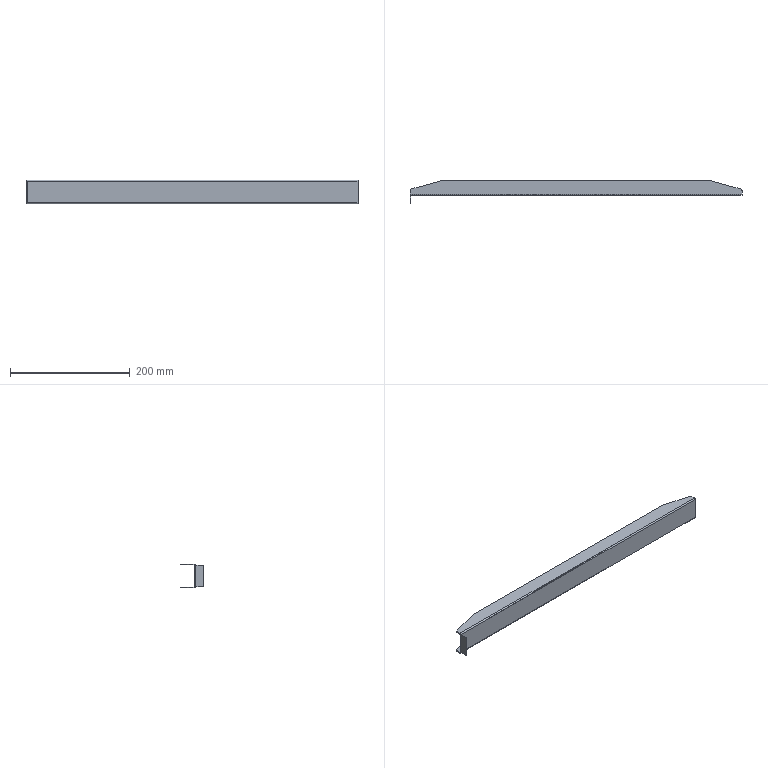Part | 1 solid | 44 faces | box 555 x 38.8 x 40 mm | volume 56167 mm3 | plane 30 | cylinder 14 | commonest cylinder face diameters 4 x8 1.48 x3 3.88 x3
STEP:
#1=CARTESIAN_POINT('',(-275.56,0.,18.06));
#2=VERTEX_POINT('',#1);
#3=CARTESIAN_POINT('',(-277.5,0.,18.06));
#4=VERTEX_POINT('',#3);
#5=CARTESIAN_POINT('',(277.5,0.,18.06));
#6=DIRECTION('',(-1.,0.,0.));
#7=VECTOR('',#6,1000.);
#8=LINE('',#5,#7);
#9=EDGE_CURVE('',#2,#4,#8,.T.);
#10=ORIENTED_EDGE('',*,*,#9,.F.);
#11=CARTESIAN_POINT('',(-277.353,-1.2,18.06));
#12=VERTEX_POINT('',#11);
#13=CARTESIAN_POINT('',(-275.56,-1.94,18.06));
#14=DIRECTION('',(0.,0.,1.));
#15=DIRECTION('',(-1.,0.,0.));
#16=AXIS2_PLACEMENT_3D('',#13,#14,#15);
#17=CIRCLE('',#16,1.94);
#18=EDGE_CURVE('',#2,#12,#17,.T.);
#19=ORIENTED_EDGE('',*,*,#18,.T.);
#20=CARTESIAN_POINT('',(-277.5,-1.2,18.06));
#21=VERTEX_POINT('',#20);
#22=CARTESIAN_POINT('',(-275.56,-1.2,18.06));
#23=DIRECTION('',(-1.,0.,0.));
#24=VECTOR('',#23,1000.);
#25=LINE('',#22,#24);
#26=EDGE_CURVE('',#12,#21,#25,.T.);
#27=ORIENTED_EDGE('',*,*,#26,.T.);
#28=CARTESIAN_POINT('',(-277.5,0.,18.06));
#29=DIRECTION('',(0.,-1.,0.));
#30=VECTOR('',#29,1000.);
#31=LINE('',#28,#30);
#32=EDGE_CURVE('',#4,#21,#31,.T.);
#33=ORIENTED_EDGE('',*,*,#32,.F.);
#34=EDGE_LOOP('',(#10,#19,#27,#33));
#35=FACE_OUTER_BOUND('',#34,.T.);
#36=CARTESIAN_POINT('',(-275.56,-1.2,18.06));
#37=DIRECTION('',(0.,0.,-1.));
#38=DIRECTION('',(-1.,0.,0.));
#39=AXIS2_PLACEMENT_3D('',#36,#37,#38);
#40=PLANE('',#39);
#41=ADVANCED_FACE('',(#35),#40,.T.);
#42=CARTESIAN_POINT('',(-277.5,-1.2,-18.06));
#43=VERTEX_POINT('',#42);
#44=CARTESIAN_POINT('',(-277.353,-1.2,-18.06));
#45=VERTEX_POINT('',#44);
#46=CARTESIAN_POINT('',(-277.5,-1.2,-18.06));
#47=DIRECTION('',(1.,0.,0.));
#48=VECTOR('',#47,1000.);
#49=LINE('',#46,#48);
#50=EDGE_CURVE('',#43,#45,#49,.T.);
#51=ORIENTED_EDGE('',*,*,#50,.T.);
#52=CARTESIAN_POINT('',(-275.56,0.,-18.06));
#53=VERTEX_POINT('',#52);
#54=CARTESIAN_POINT('',(-275.56,-1.94,-18.06));
#55=DIRECTION('',(0.,0.,-1.));
#56=DIRECTION('',(-1.,0.,0.));
#57=AXIS2_PLACEMENT_3D('',#54,#55,#56);
#58=CIRCLE('',#57,1.94);
#59=EDGE_CURVE('',#45,#53,#58,.T.);
#60=ORIENTED_EDGE('',*,*,#59,.T.);
#61=CARTESIAN_POINT('',(-277.5,0.,-18.06));
#62=VERTEX_POINT('',#61);
#63=CARTESIAN_POINT('',(-277.5,0.,-18.06));
#64=DIRECTION('',(1.,0.,0.));
#65=VECTOR('',#64,1000.);
#66=LINE('',#63,#65);
#67=EDGE_CURVE('',#62,#53,#66,.T.);
#68=ORIENTED_EDGE('',*,*,#67,.F.);
#69=CARTESIAN_POINT('',(-277.5,0.,-18.06));
#70=DIRECTION('',(0.,-1.,0.));
#71=VECTOR('',#70,1000.);
#72=LINE('',#69,#71);
#73=EDGE_CURVE('',#62,#43,#72,.T.);
#74=ORIENTED_EDGE('',*,*,#73,.T.);
#75=EDGE_LOOP('',(#51,#60,#68,#74));
#76=FACE_OUTER_BOUND('',#75,.T.);
#77=CARTESIAN_POINT('',(-277.5,-1.2,-18.06));
#78=DIRECTION('',(0.,0.,1.));
#79=DIRECTION('',(1.,0.,0.));
#80=AXIS2_PLACEMENT_3D('',#77,#78,#79);
#81=PLANE('',#80);
#82=ADVANCED_FACE('',(#76),#81,.T.);
#83=CARTESIAN_POINT('',(277.5,-1.2,18.06));
#84=VERTEX_POINT('',#83);
#85=CARTESIAN_POINT('',(-275.56,-1.2,18.06));
#86=VERTEX_POINT('',#85);
#87=CARTESIAN_POINT('',(277.5,-1.2,18.06));
#88=DIRECTION('',(-1.,0.,0.));
#89=VECTOR('',#88,1000.);
#90=LINE('',#87,#89);
#91=EDGE_CURVE('',#84,#86,#90,.T.);
#92=ORIENTED_EDGE('',*,*,#91,.T.);
#93=CARTESIAN_POINT('',(-275.56,-1.2,-18.06));
#94=VERTEX_POINT('',#93);
#95=CARTESIAN_POINT('',(-275.56,-1.2,-18.06));
#96=DIRECTION('',(0.,0.,1.));
#97=VECTOR('',#96,1000.);
#98=LINE('',#95,#97);
#99=EDGE_CURVE('',#94,#86,#98,.T.);
#100=ORIENTED_EDGE('',*,*,#99,.F.);
#101=CARTESIAN_POINT('',(277.5,-1.2,-18.06));
#102=VERTEX_POINT('',#101);
#103=CARTESIAN_POINT('',(-277.5,-1.2,-18.06));
#104=DIRECTION('',(1.,0.,0.));
#105=VECTOR('',#104,1000.);
#106=LINE('',#103,#105);
#107=EDGE_CURVE('',#94,#102,#106,.T.);
#108=ORIENTED_EDGE('',*,*,#107,.T.);
#109=CARTESIAN_POINT('',(277.5,-1.2,20.));
#110=DIRECTION('',(0.,0.,-1.));
#111=VECTOR('',#110,1000.);
#112=LINE('',#109,#111);
#113=EDGE_CURVE('',#84,#102,#112,.T.);
#114=ORIENTED_EDGE('',*,*,#113,.F.);
#115=EDGE_LOOP('',(#92,#100,#108,#114));
#116=FACE_OUTER_BOUND('',#115,.T.);
#117=CARTESIAN_POINT('',(0.,-1.2,0.));
#118=DIRECTION('',(0.,-1.,0.));
#119=DIRECTION('',(0.,0.,-1.));
#120=AXIS2_PLACEMENT_3D('',#117,#118,#119);
#121=PLANE('',#120);
#122=ADVANCED_FACE('',(#116),#121,.T.);
#123=CARTESIAN_POINT('',(-275.56,0.,-18.06));
#124=DIRECTION('',(0.,0.,1.));
#125=VECTOR('',#124,1000.);
#126=LINE('',#123,#125);
#127=EDGE_CURVE('',#53,#2,#126,.T.);
#128=ORIENTED_EDGE('',*,*,#127,.T.);
#129=CARTESIAN_POINT('',(277.5,0.,18.06));
#130=VERTEX_POINT('',#129);
#131=CARTESIAN_POINT('',(277.5,0.,18.06));
#132=DIRECTION('',(-1.,0.,0.));
#133=VECTOR('',#132,1000.);
#134=LINE('',#131,#133);
#135=EDGE_CURVE('',#130,#2,#134,.T.);
#136=ORIENTED_EDGE('',*,*,#135,.F.);
#137=CARTESIAN_POINT('',(277.5,0.,-18.06));
#138=VERTEX_POINT('',#137);
#139=CARTESIAN_POINT('',(277.5,0.,20.));
#140=DIRECTION('',(0.,0.,-1.));
#141=VECTOR('',#140,1000.);
#142=LINE('',#139,#141);
#143=EDGE_CURVE('',#130,#138,#142,.T.);
#144=ORIENTED_EDGE('',*,*,#143,.T.);
#145=CARTESIAN_POINT('',(-277.5,0.,-18.06));
#146=DIRECTION('',(1.,0.,0.));
#147=VECTOR('',#146,1000.);
#148=LINE('',#145,#147);
#149=EDGE_CURVE('',#53,#138,#148,.T.);
#150=ORIENTED_EDGE('',*,*,#149,.F.);
#151=EDGE_LOOP('',(#128,#136,#144,#150));
#152=FACE_OUTER_BOUND('',#151,.T.);
#153=CARTESIAN_POINT('',(0.,0.,0.));
#154=DIRECTION('',(0.,-1.,0.));
#155=DIRECTION('',(0.,0.,-1.));
#156=AXIS2_PLACEMENT_3D('',#153,#154,#155);
#157=PLANE('',#156);
#158=ADVANCED_FACE('',(#152),#157,.F.);
#159=CARTESIAN_POINT('',(277.5,0.,-18.06));
#160=DIRECTION('',(0.,-1.,0.));
#161=VECTOR('',#160,1000.);
#162=LINE('',#159,#161);
#163=EDGE_CURVE('',#138,#102,#162,.T.);
#164=ORIENTED_EDGE('',*,*,#163,.F.);
#165=ORIENTED_EDGE('',*,*,#143,.F.);
#166=CARTESIAN_POINT('',(277.5,0.,18.06));
#167=DIRECTION('',(0.,-1.,0.));
#168=VECTOR('',#167,1000.);
#169=LINE('',#166,#168);
#170=EDGE_CURVE('',#130,#84,#169,.T.);
#171=ORIENTED_EDGE('',*,*,#170,.T.);
#172=ORIENTED_EDGE('',*,*,#113,.T.);
#173=EDGE_LOOP('',(#164,#165,#171,#172));
#174=FACE_OUTER_BOUND('',#173,.T.);
#175=CARTESIAN_POINT('',(277.5,-1.2,20.));
#176=DIRECTION('',(1.,0.,0.));
#177=DIRECTION('',(0.,0.,-1.));
#178=AXIS2_PLACEMENT_3D('',#175,#176,#177);
#179=PLANE('',#178);
#180=ADVANCED_FACE('',(#174),#179,.T.);
#181=CARTESIAN_POINT('',(-277.5,0.74,18.8));
#182=VERTEX_POINT('',#181);
#183=CARTESIAN_POINT('',(-277.5,0.74,20.));
#184=VERTEX_POINT('',#183);
#185=CARTESIAN_POINT('',(-277.5,0.74,20.));
#186=DIRECTION('',(0.,0.,1.));
#187=VECTOR('',#186,1000.);
#188=LINE('',#185,#187);
#189=EDGE_CURVE('',#182,#184,#188,.T.);
#190=ORIENTED_EDGE('',*,*,#189,.F.);
#191=CARTESIAN_POINT('',(-277.5,0.74,18.06));
#192=DIRECTION('',(-1.,0.,0.));
#193=DIRECTION('',(0.,0.,-1.));
#194=AXIS2_PLACEMENT_3D('',#191,#192,#193);
#195=CIRCLE('',#194,0.74);
#196=EDGE_CURVE('',#4,#182,#195,.T.);
#197=ORIENTED_EDGE('',*,*,#196,.F.);
#198=ORIENTED_EDGE('',*,*,#32,.T.);
#199=CARTESIAN_POINT('',(-277.5,0.74,18.06));
#200=DIRECTION('',(-1.,0.,0.));
#201=DIRECTION('',(0.,0.,-1.));
#202=AXIS2_PLACEMENT_3D('',#199,#200,#201);
#203=CIRCLE('',#202,1.94);
#204=EDGE_CURVE('',#21,#184,#203,.T.);
#205=ORIENTED_EDGE('',*,*,#204,.T.);
#206=EDGE_LOOP('',(#190,#197,#198,#205));
#207=FACE_OUTER_BOUND('',#206,.T.);
#208=CARTESIAN_POINT('',(-277.5,0.74,18.06));
#209=DIRECTION('',(-1.,0.,0.));
#210=DIRECTION('',(0.,0.,1.));
#211=AXIS2_PLACEMENT_3D('',#208,#209,#210);
#212=PLANE('',#211);
#213=ADVANCED_FACE('',(#207),#212,.T.);
#214=CARTESIAN_POINT('',(277.5,0.74,18.8));
#215=VERTEX_POINT('',#214);
#216=CARTESIAN_POINT('',(277.5,0.74,18.06));
#217=DIRECTION('',(1.,0.,0.));
#218=DIRECTION('',(0.,0.,-1.));
#219=AXIS2_PLACEMENT_3D('',#216,#217,#218);
#220=CIRCLE('',#219,0.74);
#221=EDGE_CURVE('',#215,#130,#220,.T.);
#222=ORIENTED_EDGE('',*,*,#221,.F.);
#223=CARTESIAN_POINT('',(277.5,0.74,20.));
#224=VERTEX_POINT('',#223);
#225=CARTESIAN_POINT('',(277.5,0.74,18.8));
#226=DIRECTION('',(0.,0.,1.));
#227=VECTOR('',#226,1000.);
#228=LINE('',#225,#227);
#229=EDGE_CURVE('',#215,#224,#228,.T.);
#230=ORIENTED_EDGE('',*,*,#229,.T.);
#231=CARTESIAN_POINT('',(277.5,0.74,18.06));
#232=DIRECTION('',(1.,0.,0.));
#233=DIRECTION('',(0.,0.,-1.));
#234=AXIS2_PLACEMENT_3D('',#231,#232,#233);
#235=CIRCLE('',#234,1.94);
#236=EDGE_CURVE('',#224,#84,#235,.T.);
#237=ORIENTED_EDGE('',*,*,#236,.T.);
#238=ORIENTED_EDGE('',*,*,#170,.F.);
#239=EDGE_LOOP('',(#222,#230,#237,#238));
#240=FACE_OUTER_BOUND('',#239,.T.);
#241=CARTESIAN_POINT('',(277.5,0.74,18.06));
#242=DIRECTION('',(-1.,0.,0.));
#243=DIRECTION('',(0.,0.,1.));
#244=AXIS2_PLACEMENT_3D('',#241,#242,#243);
#245=PLANE('',#244);
#246=ADVANCED_FACE('',(#240),#245,.F.);
#247=ORIENTED_EDGE('',*,*,#91,.F.);
#248=ORIENTED_EDGE('',*,*,#236,.F.);
#249=CARTESIAN_POINT('',(0.,0.74,20.));
#250=DIRECTION('',(1.,0.,0.));
#251=VECTOR('',#250,1000.);
#252=LINE('',#249,#251);
#253=EDGE_CURVE('',#184,#224,#252,.T.);
#254=ORIENTED_EDGE('',*,*,#253,.F.);
#255=ORIENTED_EDGE('',*,*,#204,.F.);
#256=ORIENTED_EDGE('',*,*,#26,.F.);
#257=CARTESIAN_POINT('',(-275.56,-1.2,18.06));
#258=DIRECTION('',(-1.,0.,0.));
#259=VECTOR('',#258,1000.);
#260=LINE('',#257,#259);
#261=EDGE_CURVE('',#86,#12,#260,.T.);
#262=ORIENTED_EDGE('',*,*,#261,.F.);
#263=EDGE_LOOP('',(#247,#248,#254,#255,#256,#262));
#264=FACE_OUTER_BOUND('',#263,.T.);
#265=CARTESIAN_POINT('',(277.5,0.74,18.06));
#266=DIRECTION('',(1.,0.,0.));
#267=DIRECTION('',(0.,0.,1.));
#268=AXIS2_PLACEMENT_3D('',#265,#266,#267);
#269=CYLINDRICAL_SURFACE('',#268,1.94);
#270=ADVANCED_FACE('',(#264),#269,.T.);
#271=ORIENTED_EDGE('',*,*,#135,.T.);
#272=ORIENTED_EDGE('',*,*,#9,.T.);
#273=ORIENTED_EDGE('',*,*,#196,.T.);
#274=CARTESIAN_POINT('',(-277.5,0.74,18.8));
#275=DIRECTION('',(1.,0.,0.));
#276=VECTOR('',#275,1000.);
#277=LINE('',#274,#276);
#278=EDGE_CURVE('',#182,#215,#277,.T.);
#279=ORIENTED_EDGE('',*,*,#278,.T.);
#280=ORIENTED_EDGE('',*,*,#221,.T.);
#281=EDGE_LOOP('',(#271,#272,#273,#279,#280));
#282=FACE_OUTER_BOUND('',#281,.T.);
#283=CARTESIAN_POINT('',(277.5,0.74,18.06));
#284=DIRECTION('',(1.,0.,0.));
#285=DIRECTION('',(0.,0.,1.));
#286=AXIS2_PLACEMENT_3D('',#283,#284,#285);
#287=CYLINDRICAL_SURFACE('',#286,0.74);
#288=ADVANCED_FACE('',(#282),#287,.F.);
#289=CARTESIAN_POINT('',(277.5,7.272,18.8));
#290=VERTEX_POINT('',#289);
#291=CARTESIAN_POINT('',(277.5,0.,18.8));
#292=DIRECTION('',(0.,-1.,0.));
#293=VECTOR('',#292,1000.);
#294=LINE('',#291,#293);
#295=EDGE_CURVE('',#290,#215,#294,.T.);
#296=ORIENTED_EDGE('',*,*,#295,.F.);
#297=CARTESIAN_POINT('',(277.5,7.272,20.));
#298=VERTEX_POINT('',#297);
#299=CARTESIAN_POINT('',(277.5,7.272,20.));
#300=DIRECTION('',(0.,0.,1.));
#301=VECTOR('',#300,1000.);
#302=LINE('',#299,#301);
#303=EDGE_CURVE('',#290,#298,#302,.T.);
#304=ORIENTED_EDGE('',*,*,#303,.T.);
#305=CARTESIAN_POINT('',(277.5,0.,20.));
#306=DIRECTION('',(0.,-1.,0.));
#307=VECTOR('',#306,1000.);
#308=LINE('',#305,#307);
#309=EDGE_CURVE('',#298,#224,#308,.T.);
#310=ORIENTED_EDGE('',*,*,#309,.T.);
#311=ORIENTED_EDGE('',*,*,#229,.F.);
#312=EDGE_LOOP('',(#296,#304,#310,#311));
#313=FACE_OUTER_BOUND('',#312,.T.);
#314=CARTESIAN_POINT('',(277.5,0.,20.));
#315=DIRECTION('',(1.,0.,0.));
#316=DIRECTION('',(0.,0.,-1.));
#317=AXIS2_PLACEMENT_3D('',#314,#315,#316);
#318=PLANE('',#317);
#319=ADVANCED_FACE('',(#313),#318,.T.);
#320=CARTESIAN_POINT('',(-277.5,7.272,20.));
#321=VERTEX_POINT('',#320);
#322=CARTESIAN_POINT('',(-277.5,23.8,20.));
#323=DIRECTION('',(0.,1.,0.));
#324=VECTOR('',#323,1000.);
#325=LINE('',#322,#324);
#326=EDGE_CURVE('',#184,#321,#325,.T.);
#327=ORIENTED_EDGE('',*,*,#326,.T.);
#328=CARTESIAN_POINT('',(-277.5,7.272,18.8));
#329=VERTEX_POINT('',#328);
#330=CARTESIAN_POINT('',(-277.5,7.272,20.));
#331=DIRECTION('',(0.,0.,-1.));
#332=VECTOR('',#331,1000.);
#333=LINE('',#330,#332);
#334=EDGE_CURVE('',#321,#329,#333,.T.);
#335=ORIENTED_EDGE('',*,*,#334,.T.);
#336=CARTESIAN_POINT('',(-277.5,0.,18.8));
#337=DIRECTION('',(0.,1.,0.));
#338=VECTOR('',#337,1000.);
#339=LINE('',#336,#338);
#340=EDGE_CURVE('',#182,#329,#339,.T.);
#341=ORIENTED_EDGE('',*,*,#340,.F.);
#342=ORIENTED_EDGE('',*,*,#189,.T.);
#343=EDGE_LOOP('',(#327,#335,#341,#342));
#344=FACE_OUTER_BOUND('',#343,.T.);
#345=CARTESIAN_POINT('',(-277.5,23.8,20.));
#346=DIRECTION('',(-1.,0.,0.));
#347=DIRECTION('',(0.,0.,1.));
#348=AXIS2_PLACEMENT_3D('',#345,#346,#347);
#349=PLANE('',#348);
#350=ADVANCED_FACE('',(#344),#349,.T.);
#351=CARTESIAN_POINT('',(-222.758,23.73,20.));
#352=VERTEX_POINT('',#351);
#353=CARTESIAN_POINT('',(-276.026,9.202,20.));
#354=VERTEX_POINT('',#353);
#355=CARTESIAN_POINT('',(-21.445,78.633,20.));
#356=DIRECTION('',(-0.9648,-0.2631,0.));
#357=VECTOR('',#356,1000.);
#358=LINE('',#355,#357);
#359=EDGE_CURVE('',#352,#354,#358,.T.);
#360=ORIENTED_EDGE('',*,*,#359,.T.);
#361=CARTESIAN_POINT('',(-275.5,7.272,20.));
#362=DIRECTION('',(0.,0.,1.));
#363=DIRECTION('',(0.,-1.,0.));
#364=AXIS2_PLACEMENT_3D('',#361,#362,#363);
#365=CIRCLE('',#364,2.);
#366=EDGE_CURVE('',#354,#321,#365,.T.);
#367=ORIENTED_EDGE('',*,*,#366,.T.);
#368=ORIENTED_EDGE('',*,*,#326,.F.);
#369=ORIENTED_EDGE('',*,*,#253,.T.);
#370=ORIENTED_EDGE('',*,*,#309,.F.);
#371=CARTESIAN_POINT('',(276.026,9.202,20.));
#372=VERTEX_POINT('',#371);
#373=CARTESIAN_POINT('',(275.5,7.272,20.));
#374=DIRECTION('',(0.,0.,1.));
#375=DIRECTION('',(0.,-1.,0.));
#376=AXIS2_PLACEMENT_3D('',#373,#374,#375);
#377=CIRCLE('',#376,2.);
#378=EDGE_CURVE('',#298,#372,#377,.T.);
#379=ORIENTED_EDGE('',*,*,#378,.T.);
#380=CARTESIAN_POINT('',(222.758,23.73,20.));
#381=VERTEX_POINT('',#380);
#382=CARTESIAN_POINT('',(21.445,78.633,20.));
#383=DIRECTION('',(-0.9648,0.2631,0.));
#384=VECTOR('',#383,1000.);
#385=LINE('',#382,#384);
#386=EDGE_CURVE('',#372,#381,#385,.T.);
#387=ORIENTED_EDGE('',*,*,#386,.T.);
#388=CARTESIAN_POINT('',(222.232,23.8,20.));
#389=VERTEX_POINT('',#388);
#390=CARTESIAN_POINT('',(222.232,21.8,20.));
#391=DIRECTION('',(0.,0.,1.));
#392=DIRECTION('',(0.,-1.,0.));
#393=AXIS2_PLACEMENT_3D('',#390,#391,#392);
#394=CIRCLE('',#393,2.);
#395=EDGE_CURVE('',#381,#389,#394,.T.);
#396=ORIENTED_EDGE('',*,*,#395,.T.);
#397=CARTESIAN_POINT('',(-222.232,23.8,20.));
#398=VERTEX_POINT('',#397);
#399=CARTESIAN_POINT('',(277.5,23.8,20.));
#400=DIRECTION('',(1.,0.,0.));
#401=VECTOR('',#400,1000.);
#402=LINE('',#399,#401);
#403=EDGE_CURVE('',#398,#389,#402,.T.);
#404=ORIENTED_EDGE('',*,*,#403,.F.);
#405=CARTESIAN_POINT('',(-222.232,21.8,20.));
#406=DIRECTION('',(0.,0.,1.));
#407=DIRECTION('',(0.,-1.,0.));
#408=AXIS2_PLACEMENT_3D('',#405,#406,#407);
#409=CIRCLE('',#408,2.);
#410=EDGE_CURVE('',#398,#352,#409,.T.);
#411=ORIENTED_EDGE('',*,*,#410,.T.);
#412=EDGE_LOOP('',(#360,#367,#368,#369,#370,#379,#387,#396,#404,#411));
#413=FACE_OUTER_BOUND('',#412,.T.);
#414=CARTESIAN_POINT('',(0.,0.,20.));
#415=DIRECTION('',(0.,0.,1.));
#416=DIRECTION('',(0.,-1.,0.));
#417=AXIS2_PLACEMENT_3D('',#414,#415,#416);
#418=PLANE('',#417);
#419=ADVANCED_FACE('',(#413),#418,.T.);
#420=ORIENTED_EDGE('',*,*,#340,.T.);
#421=CARTESIAN_POINT('',(-276.026,9.202,18.8));
#422=VERTEX_POINT('',#421);
#423=CARTESIAN_POINT('',(-275.5,7.272,18.8));
#424=DIRECTION('',(0.,0.,-1.));
#425=DIRECTION('',(0.,-1.,0.));
#426=AXIS2_PLACEMENT_3D('',#423,#424,#425);
#427=CIRCLE('',#426,2.);
#428=EDGE_CURVE('',#329,#422,#427,.T.);
#429=ORIENTED_EDGE('',*,*,#428,.T.);
#430=CARTESIAN_POINT('',(-222.758,23.73,18.8));
#431=VERTEX_POINT('',#430);
#432=CARTESIAN_POINT('',(-277.5,8.8,18.8));
#433=DIRECTION('',(0.9648,0.2631,0.));
#434=VECTOR('',#433,1000.);
#435=LINE('',#432,#434);
#436=EDGE_CURVE('',#422,#431,#435,.T.);
#437=ORIENTED_EDGE('',*,*,#436,.T.);
#438=CARTESIAN_POINT('',(-222.232,23.8,18.8));
#439=VERTEX_POINT('',#438);
#440=CARTESIAN_POINT('',(-222.232,21.8,18.8));
#441=DIRECTION('',(0.,0.,-1.));
#442=DIRECTION('',(0.,-1.,0.));
#443=AXIS2_PLACEMENT_3D('',#440,#441,#442);
#444=CIRCLE('',#443,2.);
#445=EDGE_CURVE('',#431,#439,#444,.T.);
#446=ORIENTED_EDGE('',*,*,#445,.T.);
#447=CARTESIAN_POINT('',(222.232,23.8,18.8));
#448=VERTEX_POINT('',#447);
#449=CARTESIAN_POINT('',(0.,23.8,18.8));
#450=DIRECTION('',(1.,0.,0.));
#451=VECTOR('',#450,1000.);
#452=LINE('',#449,#451);
#453=EDGE_CURVE('',#439,#448,#452,.T.);
#454=ORIENTED_EDGE('',*,*,#453,.T.);
#455=CARTESIAN_POINT('',(222.758,23.73,18.8));
#456=VERTEX_POINT('',#455);
#457=CARTESIAN_POINT('',(222.232,21.8,18.8));
#458=DIRECTION('',(0.,0.,-1.));
#459=DIRECTION('',(0.,-1.,0.));
#460=AXIS2_PLACEMENT_3D('',#457,#458,#459);
#461=CIRCLE('',#460,2.);
#462=EDGE_CURVE('',#448,#456,#461,.T.);
#463=ORIENTED_EDGE('',*,*,#462,.T.);
#464=CARTESIAN_POINT('',(276.026,9.202,18.8));
#465=VERTEX_POINT('',#464);
#466=CARTESIAN_POINT('',(222.5,23.8,18.8));
#467=DIRECTION('',(0.9648,-0.2631,0.));
#468=VECTOR('',#467,1000.);
#469=LINE('',#466,#468);
#470=EDGE_CURVE('',#456,#465,#469,.T.);
#471=ORIENTED_EDGE('',*,*,#470,.T.);
#472=CARTESIAN_POINT('',(275.5,7.272,18.8));
#473=DIRECTION('',(0.,0.,-1.));
#474=DIRECTION('',(0.,-1.,0.));
#475=AXIS2_PLACEMENT_3D('',#472,#473,#474);
#476=CIRCLE('',#475,2.);
#477=EDGE_CURVE('',#465,#290,#476,.T.);
#478=ORIENTED_EDGE('',*,*,#477,.T.);
#479=ORIENTED_EDGE('',*,*,#295,.T.);
#480=ORIENTED_EDGE('',*,*,#278,.F.);
#481=EDGE_LOOP('',(#420,#429,#437,#446,#454,#463,#471,#478,#479,#480));
#482=FACE_OUTER_BOUND('',#481,.T.);
#483=CARTESIAN_POINT('',(0.,0.,18.8));
#484=DIRECTION('',(0.,0.,1.));
#485=DIRECTION('',(0.,-1.,0.));
#486=AXIS2_PLACEMENT_3D('',#483,#484,#485);
#487=PLANE('',#486);
#488=ADVANCED_FACE('',(#482),#487,.F.);
#489=ORIENTED_EDGE('',*,*,#453,.F.);
#490=CARTESIAN_POINT('',(-222.232,23.8,20.));
#491=DIRECTION('',(0.,0.,1.));
#492=VECTOR('',#491,1000.);
#493=LINE('',#490,#492);
#494=EDGE_CURVE('',#439,#398,#493,.T.);
#495=ORIENTED_EDGE('',*,*,#494,.T.);
#496=ORIENTED_EDGE('',*,*,#403,.T.);
#497=CARTESIAN_POINT('',(222.232,23.8,20.));
#498=DIRECTION('',(0.,0.,-1.));
#499=VECTOR('',#498,1000.);
#500=LINE('',#497,#499);
#501=EDGE_CURVE('',#389,#448,#500,.T.);
#502=ORIENTED_EDGE('',*,*,#501,.T.);
#503=EDGE_LOOP('',(#489,#495,#496,#502));
#504=FACE_OUTER_BOUND('',#503,.T.);
#505=CARTESIAN_POINT('',(277.5,23.8,20.));
#506=DIRECTION('',(0.,1.,0.));
#507=DIRECTION('',(0.,0.,1.));
#508=AXIS2_PLACEMENT_3D('',#505,#506,#507);
#509=PLANE('',#508);
#510=ADVANCED_FACE('',(#504),#509,.T.);
#511=CARTESIAN_POINT('',(277.5,0.74,-18.8));
#512=VERTEX_POINT('',#511);
#513=CARTESIAN_POINT('',(277.5,0.74,-20.));
#514=VERTEX_POINT('',#513);
#515=CARTESIAN_POINT('',(277.5,0.74,-20.));
#516=DIRECTION('',(0.,0.,-1.));
#517=VECTOR('',#516,1000.);
#518=LINE('',#515,#517);
#519=EDGE_CURVE('',#512,#514,#518,.T.);
#520=ORIENTED_EDGE('',*,*,#519,.F.);
#521=CARTESIAN_POINT('',(277.5,0.74,-18.06));
#522=DIRECTION('',(1.,0.,0.));
#523=DIRECTION('',(0.,0.,1.));
#524=AXIS2_PLACEMENT_3D('',#521,#522,#523);
#525=CIRCLE('',#524,0.74);
#526=EDGE_CURVE('',#138,#512,#525,.T.);
#527=ORIENTED_EDGE('',*,*,#526,.F.);
#528=ORIENTED_EDGE('',*,*,#163,.T.);
#529=CARTESIAN_POINT('',(277.5,0.74,-18.06));
#530=DIRECTION('',(1.,0.,0.));
#531=DIRECTION('',(0.,0.,1.));
#532=AXIS2_PLACEMENT_3D('',#529,#530,#531);
#533=CIRCLE('',#532,1.94);
#534=EDGE_CURVE('',#102,#514,#533,.T.);
#535=ORIENTED_EDGE('',*,*,#534,.T.);
#536=EDGE_LOOP('',(#520,#527,#528,#535));
#537=FACE_OUTER_BOUND('',#536,.T.);
#538=CARTESIAN_POINT('',(277.5,0.74,-18.06));
#539=DIRECTION('',(1.,0.,0.));
#540=DIRECTION('',(0.,0.,-1.));
#541=AXIS2_PLACEMENT_3D('',#538,#539,#540);
#542=PLANE('',#541);
#543=ADVANCED_FACE('',(#537),#542,.T.);
#544=CARTESIAN_POINT('',(-277.5,0.74,-18.8));
#545=VERTEX_POINT('',#544);
#546=CARTESIAN_POINT('',(-277.5,0.74,-18.06));
#547=DIRECTION('',(-1.,0.,0.));
#548=DIRECTION('',(0.,0.,1.));
#549=AXIS2_PLACEMENT_3D('',#546,#547,#548);
#550=CIRCLE('',#549,0.74);
#551=EDGE_CURVE('',#545,#62,#550,.T.);
#552=ORIENTED_EDGE('',*,*,#551,.F.);
#553=CARTESIAN_POINT('',(-277.5,0.74,-20.));
#554=VERTEX_POINT('',#553);
#555=CARTESIAN_POINT('',(-277.5,0.74,-18.8));
#556=DIRECTION('',(0.,0.,-1.));
#557=VECTOR('',#556,1000.);
#558=LINE('',#555,#557);
#559=EDGE_CURVE('',#545,#554,#558,.T.);
#560=ORIENTED_EDGE('',*,*,#559,.T.);
#561=CARTESIAN_POINT('',(-277.5,0.74,-18.06));
#562=DIRECTION('',(-1.,0.,0.));
#563=DIRECTION('',(0.,0.,1.));
#564=AXIS2_PLACEMENT_3D('',#561,#562,#563);
#565=CIRCLE('',#564,1.94);
#566=EDGE_CURVE('',#554,#43,#565,.T.);
#567=ORIENTED_EDGE('',*,*,#566,.T.);
#568=ORIENTED_EDGE('',*,*,#73,.F.);
#569=EDGE_LOOP('',(#552,#560,#567,#568));
#570=FACE_OUTER_BOUND('',#569,.T.);
#571=CARTESIAN_POINT('',(-277.5,0.74,-18.06));
#572=DIRECTION('',(1.,0.,0.));
#573=DIRECTION('',(0.,0.,-1.));
#574=AXIS2_PLACEMENT_3D('',#571,#572,#573);
#575=PLANE('',#574);
#576=ADVANCED_FACE('',(#570),#575,.F.);
#577=ORIENTED_EDGE('',*,*,#50,.F.);
#578=ORIENTED_EDGE('',*,*,#566,.F.);
#579=CARTESIAN_POINT('',(277.5,0.74,-20.));
#580=DIRECTION('',(1.,0.,0.));
#581=VECTOR('',#580,1000.);
#582=LINE('',#579,#581);
#583=EDGE_CURVE('',#554,#514,#582,.T.);
#584=ORIENTED_EDGE('',*,*,#583,.T.);
#585=ORIENTED_EDGE('',*,*,#534,.F.);
#586=ORIENTED_EDGE('',*,*,#107,.F.);
#587=CARTESIAN_POINT('',(-277.5,-1.2,-18.06));
#588=DIRECTION('',(1.,0.,0.));
#589=VECTOR('',#588,1000.);
#590=LINE('',#587,#589);
#591=EDGE_CURVE('',#45,#94,#590,.T.);
#592=ORIENTED_EDGE('',*,*,#591,.F.);
#593=EDGE_LOOP('',(#577,#578,#584,#585,#586,#592));
#594=FACE_OUTER_BOUND('',#593,.T.);
#595=CARTESIAN_POINT('',(-277.5,0.74,-18.06));
#596=DIRECTION('',(-1.,0.,0.));
#597=DIRECTION('',(0.,0.,-1.));
#598=AXIS2_PLACEMENT_3D('',#595,#596,#597);
#599=CYLINDRICAL_SURFACE('',#598,1.94);
#600=ADVANCED_FACE('',(#594),#599,.T.);
#601=ORIENTED_EDGE('',*,*,#67,.T.);
#602=ORIENTED_EDGE('',*,*,#149,.T.);
#603=ORIENTED_EDGE('',*,*,#526,.T.);
#604=CARTESIAN_POINT('',(277.5,0.74,-18.8));
#605=DIRECTION('',(-1.,0.,0.));
#606=VECTOR('',#605,1000.);
#607=LINE('',#604,#606);
#608=EDGE_CURVE('',#512,#545,#607,.T.);
#609=ORIENTED_EDGE('',*,*,#608,.T.);
#610=ORIENTED_EDGE('',*,*,#551,.T.);
#611=EDGE_LOOP('',(#601,#602,#603,#609,#610));
#612=FACE_OUTER_BOUND('',#611,.T.);
#613=CARTESIAN_POINT('',(-277.5,0.74,-18.06));
#614=DIRECTION('',(-1.,0.,0.));
#615=DIRECTION('',(0.,0.,-1.));
#616=AXIS2_PLACEMENT_3D('',#613,#614,#615);
#617=CYLINDRICAL_SURFACE('',#616,0.74);
#618=ADVANCED_FACE('',(#612),#617,.F.);
#619=CARTESIAN_POINT('',(277.5,7.272,-20.));
#620=VERTEX_POINT('',#619);
#621=CARTESIAN_POINT('',(277.5,0.,-20.));
#622=DIRECTION('',(0.,1.,0.));
#623=VECTOR('',#622,1000.);
#624=LINE('',#621,#623);
#625=EDGE_CURVE('',#514,#620,#624,.T.);
#626=ORIENTED_EDGE('',*,*,#625,.T.);
#627=CARTESIAN_POINT('',(277.5,7.272,-18.8));
#628=VERTEX_POINT('',#627);
#629=CARTESIAN_POINT('',(277.5,7.272,-20.));
#630=DIRECTION('',(0.,0.,1.));
#631=VECTOR('',#630,1000.);
#632=LINE('',#629,#631);
#633=EDGE_CURVE('',#620,#628,#632,.T.);
#634=ORIENTED_EDGE('',*,*,#633,.T.);
#635=CARTESIAN_POINT('',(277.5,0.,-18.8));
#636=DIRECTION('',(0.,1.,0.));
#637=VECTOR('',#636,1000.);
#638=LINE('',#635,#637);
#639=EDGE_CURVE('',#512,#628,#638,.T.);
#640=ORIENTED_EDGE('',*,*,#639,.F.);
#641=ORIENTED_EDGE('',*,*,#519,.T.);
#642=EDGE_LOOP('',(#626,#634,#640,#641));
#643=FACE_OUTER_BOUND('',#642,.T.);
#644=CARTESIAN_POINT('',(277.5,0.,-20.));
#645=DIRECTION('',(1.,0.,0.));
#646=DIRECTION('',(0.,0.,-1.));
#647=AXIS2_PLACEMENT_3D('',#644,#645,#646);
#648=PLANE('',#647);
#649=ADVANCED_FACE('',(#643),#648,.T.);
#650=CARTESIAN_POINT('',(-277.5,7.272,-18.8));
#651=VERTEX_POINT('',#650);
#652=CARTESIAN_POINT('',(-277.5,0.,-18.8));
#653=DIRECTION('',(0.,-1.,0.));
#654=VECTOR('',#653,1000.);
#655=LINE('',#652,#654);
#656=EDGE_CURVE('',#651,#545,#655,.T.);
#657=ORIENTED_EDGE('',*,*,#656,.F.);
#658=CARTESIAN_POINT('',(-277.5,7.272,-20.));
#659=VERTEX_POINT('',#658);
#660=CARTESIAN_POINT('',(-277.5,7.272,-20.));
#661=DIRECTION('',(0.,0.,-1.));
#662=VECTOR('',#661,1000.);
#663=LINE('',#660,#662);
#664=EDGE_CURVE('',#651,#659,#663,.T.);
#665=ORIENTED_EDGE('',*,*,#664,.T.);
#666=CARTESIAN_POINT('',(-277.5,23.8,-20.));
#667=DIRECTION('',(0.,-1.,0.));
#668=VECTOR('',#667,1000.);
#669=LINE('',#666,#668);
#670=EDGE_CURVE('',#659,#554,#669,.T.);
#671=ORIENTED_EDGE('',*,*,#670,.T.);
#672=ORIENTED_EDGE('',*,*,#559,.F.);
#673=EDGE_LOOP('',(#657,#665,#671,#672));
#674=FACE_OUTER_BOUND('',#673,.T.);
#675=CARTESIAN_POINT('',(-277.5,23.8,-20.));
#676=DIRECTION('',(-1.,0.,0.));
#677=DIRECTION('',(0.,0.,1.));
#678=AXIS2_PLACEMENT_3D('',#675,#676,#677);
#679=PLANE('',#678);
#680=ADVANCED_FACE('',(#674),#679,.T.);
#681=CARTESIAN_POINT('',(222.758,23.73,-20.));
#682=VERTEX_POINT('',#681);
#683=CARTESIAN_POINT('',(276.026,9.202,-20.));
#684=VERTEX_POINT('',#683);
#685=CARTESIAN_POINT('',(277.5,8.8,-20.));
#686=DIRECTION('',(0.9648,-0.2631,0.));
#687=VECTOR('',#686,1000.);
#688=LINE('',#685,#687);
#689=EDGE_CURVE('',#682,#684,#688,.T.);
#690=ORIENTED_EDGE('',*,*,#689,.T.);
#691=CARTESIAN_POINT('',(275.5,7.272,-20.));
#692=DIRECTION('',(0.,0.,-1.));
#693=DIRECTION('',(1.,0.,0.));
#694=AXIS2_PLACEMENT_3D('',#691,#692,#693);
#695=CIRCLE('',#694,2.);
#696=EDGE_CURVE('',#684,#620,#695,.T.);
#697=ORIENTED_EDGE('',*,*,#696,.T.);
#698=ORIENTED_EDGE('',*,*,#625,.F.);
#699=ORIENTED_EDGE('',*,*,#583,.F.);
#700=ORIENTED_EDGE('',*,*,#670,.F.);
#701=CARTESIAN_POINT('',(-276.026,9.202,-20.));
#702=VERTEX_POINT('',#701);
#703=CARTESIAN_POINT('',(-275.5,7.272,-20.));
#704=DIRECTION('',(0.,0.,-1.));
#705=DIRECTION('',(1.,0.,0.));
#706=AXIS2_PLACEMENT_3D('',#703,#704,#705);
#707=CIRCLE('',#706,2.);
#708=EDGE_CURVE('',#659,#702,#707,.T.);
#709=ORIENTED_EDGE('',*,*,#708,.T.);
#710=CARTESIAN_POINT('',(-222.758,23.73,-20.));
#711=VERTEX_POINT('',#710);
#712=CARTESIAN_POINT('',(-222.5,23.8,-20.));
#713=DIRECTION('',(0.9648,0.2631,0.));
#714=VECTOR('',#713,1000.);
#715=LINE('',#712,#714);
#716=EDGE_CURVE('',#702,#711,#715,.T.);
#717=ORIENTED_EDGE('',*,*,#716,.T.);
#718=CARTESIAN_POINT('',(-222.232,23.8,-20.));
#719=VERTEX_POINT('',#718);
#720=CARTESIAN_POINT('',(-222.232,21.8,-20.));
#721=DIRECTION('',(0.,0.,-1.));
#722=DIRECTION('',(1.,0.,0.));
#723=AXIS2_PLACEMENT_3D('',#720,#721,#722);
#724=CIRCLE('',#723,2.);
#725=EDGE_CURVE('',#711,#719,#724,.T.);
#726=ORIENTED_EDGE('',*,*,#725,.T.);
#727=CARTESIAN_POINT('',(222.232,23.8,-20.));
#728=VERTEX_POINT('',#727);
#729=CARTESIAN_POINT('',(277.5,23.8,-20.));
#730=DIRECTION('',(-1.,0.,0.));
#731=VECTOR('',#730,1000.);
#732=LINE('',#729,#731);
#733=EDGE_CURVE('',#728,#719,#732,.T.);
#734=ORIENTED_EDGE('',*,*,#733,.F.);
#735=CARTESIAN_POINT('',(222.232,21.8,-20.));
#736=DIRECTION('',(0.,0.,-1.));
#737=DIRECTION('',(1.,0.,0.));
#738=AXIS2_PLACEMENT_3D('',#735,#736,#737);
#739=CIRCLE('',#738,2.);
#740=EDGE_CURVE('',#728,#682,#739,.T.);
#741=ORIENTED_EDGE('',*,*,#740,.T.);
#742=EDGE_LOOP('',(#690,#697,#698,#699,#700,#709,#717,#726,#734,#741));
#743=FACE_OUTER_BOUND('',#742,.T.);
#744=CARTESIAN_POINT('',(0.,0.,-20.));
#745=DIRECTION('',(0.,0.,1.));
#746=DIRECTION('',(1.,0.,0.));
#747=AXIS2_PLACEMENT_3D('',#744,#745,#746);
#748=PLANE('',#747);
#749=ADVANCED_FACE('',(#743),#748,.F.);
#750=ORIENTED_EDGE('',*,*,#639,.T.);
#751=CARTESIAN_POINT('',(276.026,9.202,-18.8));
#752=VERTEX_POINT('',#751);
#753=CARTESIAN_POINT('',(275.5,7.272,-18.8));
#754=DIRECTION('',(0.,0.,1.));
#755=DIRECTION('',(1.,0.,0.));
#756=AXIS2_PLACEMENT_3D('',#753,#754,#755);
#757=CIRCLE('',#756,2.);
#758=EDGE_CURVE('',#628,#752,#757,.T.);
#759=ORIENTED_EDGE('',*,*,#758,.T.);
#760=CARTESIAN_POINT('',(222.758,23.73,-18.8));
#761=VERTEX_POINT('',#760);
#762=CARTESIAN_POINT('',(21.445,78.633,-18.8));
#763=DIRECTION('',(-0.9648,0.2631,0.));
#764=VECTOR('',#763,1000.);
#765=LINE('',#762,#764);
#766=EDGE_CURVE('',#752,#761,#765,.T.);
#767=ORIENTED_EDGE('',*,*,#766,.T.);
#768=CARTESIAN_POINT('',(222.232,23.8,-18.8));
#769=VERTEX_POINT('',#768);
#770=CARTESIAN_POINT('',(222.232,21.8,-18.8));
#771=DIRECTION('',(0.,0.,1.));
#772=DIRECTION('',(1.,0.,0.));
#773=AXIS2_PLACEMENT_3D('',#770,#771,#772);
#774=CIRCLE('',#773,2.);
#775=EDGE_CURVE('',#761,#769,#774,.T.);
#776=ORIENTED_EDGE('',*,*,#775,.T.);
#777=CARTESIAN_POINT('',(-222.232,23.8,-18.8));
#778=VERTEX_POINT('',#777);
#779=CARTESIAN_POINT('',(0.,23.8,-18.8));
#780=DIRECTION('',(-1.,0.,0.));
#781=VECTOR('',#780,1000.);
#782=LINE('',#779,#781);
#783=EDGE_CURVE('',#769,#778,#782,.T.);
#784=ORIENTED_EDGE('',*,*,#783,.T.);
#785=CARTESIAN_POINT('',(-222.758,23.73,-18.8));
#786=VERTEX_POINT('',#785);
#787=CARTESIAN_POINT('',(-222.232,21.8,-18.8));
#788=DIRECTION('',(0.,0.,1.));
#789=DIRECTION('',(1.,0.,0.));
#790=AXIS2_PLACEMENT_3D('',#787,#788,#789);
#791=CIRCLE('',#790,2.);
#792=EDGE_CURVE('',#778,#786,#791,.T.);
#793=ORIENTED_EDGE('',*,*,#792,.T.);
#794=CARTESIAN_POINT('',(-276.026,9.202,-18.8));
#795=VERTEX_POINT('',#794);
#796=CARTESIAN_POINT('',(-21.445,78.633,-18.8));
#797=DIRECTION('',(-0.9648,-0.2631,0.));
#798=VECTOR('',#797,1000.);
#799=LINE('',#796,#798);
#800=EDGE_CURVE('',#786,#795,#799,.T.);
#801=ORIENTED_EDGE('',*,*,#800,.T.);
#802=CARTESIAN_POINT('',(-275.5,7.272,-18.8));
#803=DIRECTION('',(0.,0.,1.));
#804=DIRECTION('',(1.,0.,0.));
#805=AXIS2_PLACEMENT_3D('',#802,#803,#804);
#806=CIRCLE('',#805,2.);
#807=EDGE_CURVE('',#795,#651,#806,.T.);
#808=ORIENTED_EDGE('',*,*,#807,.T.);
#809=ORIENTED_EDGE('',*,*,#656,.T.);
#810=ORIENTED_EDGE('',*,*,#608,.F.);
#811=EDGE_LOOP('',(#750,#759,#767,#776,#784,#793,#801,#808,#809,#810));
#812=FACE_OUTER_BOUND('',#811,.T.);
#813=CARTESIAN_POINT('',(0.,0.,-18.8));
#814=DIRECTION('',(0.,0.,1.));
#815=DIRECTION('',(1.,0.,0.));
#816=AXIS2_PLACEMENT_3D('',#813,#814,#815);
#817=PLANE('',#816);
#818=ADVANCED_FACE('',(#812),#817,.T.);
#819=ORIENTED_EDGE('',*,*,#783,.F.);
#820=CARTESIAN_POINT('',(222.232,23.8,-20.));
#821=DIRECTION('',(0.,0.,-1.));
#822=VECTOR('',#821,1000.);
#823=LINE('',#820,#822);
#824=EDGE_CURVE('',#769,#728,#823,.T.);
#825=ORIENTED_EDGE('',*,*,#824,.T.);
#826=ORIENTED_EDGE('',*,*,#733,.T.);
#827=CARTESIAN_POINT('',(-222.232,23.8,-20.));
#828=DIRECTION('',(0.,0.,1.));
#829=VECTOR('',#828,1000.);
#830=LINE('',#827,#829);
#831=EDGE_CURVE('',#719,#778,#830,.T.);
#832=ORIENTED_EDGE('',*,*,#831,.T.);
#833=EDGE_LOOP('',(#819,#825,#826,#832));
#834=FACE_OUTER_BOUND('',#833,.T.);
#835=CARTESIAN_POINT('',(277.5,23.8,-20.));
#836=DIRECTION('',(0.,1.,0.));
#837=DIRECTION('',(-1.,0.,0.));
#838=AXIS2_PLACEMENT_3D('',#835,#836,#837);
#839=PLANE('',#838);
#840=ADVANCED_FACE('',(#834),#839,.T.);
#841=ORIENTED_EDGE('',*,*,#470,.F.);
#842=CARTESIAN_POINT('',(222.758,23.73,20.));
#843=DIRECTION('',(0.,0.,1.));
#844=VECTOR('',#843,1000.);
#845=LINE('',#842,#844);
#846=EDGE_CURVE('',#456,#381,#845,.T.);
#847=ORIENTED_EDGE('',*,*,#846,.T.);
#848=ORIENTED_EDGE('',*,*,#386,.F.);
#849=CARTESIAN_POINT('',(276.026,9.202,20.));
#850=DIRECTION('',(0.,0.,-1.));
#851=VECTOR('',#850,1000.);
#852=LINE('',#849,#851);
#853=EDGE_CURVE('',#372,#465,#852,.T.);
#854=ORIENTED_EDGE('',*,*,#853,.T.);
#855=EDGE_LOOP('',(#841,#847,#848,#854));
#856=FACE_OUTER_BOUND('',#855,.T.);
#857=CARTESIAN_POINT('',(222.5,23.8,20.));
#858=DIRECTION('',(-0.2631,-0.9648,0.));
#859=DIRECTION('',(0.,0.,-1.));
#860=AXIS2_PLACEMENT_3D('',#857,#858,#859);
#861=PLANE('',#860);
#862=ADVANCED_FACE('',(#856),#861,.F.);
#863=ORIENTED_EDGE('',*,*,#766,.F.);
#864=CARTESIAN_POINT('',(276.026,9.202,-20.));
#865=DIRECTION('',(0.,0.,-1.));
#866=VECTOR('',#865,1000.);
#867=LINE('',#864,#866);
#868=EDGE_CURVE('',#752,#684,#867,.T.);
#869=ORIENTED_EDGE('',*,*,#868,.T.);
#870=ORIENTED_EDGE('',*,*,#689,.F.);
#871=CARTESIAN_POINT('',(222.758,23.73,-20.));
#872=DIRECTION('',(0.,0.,1.));
#873=VECTOR('',#872,1000.);
#874=LINE('',#871,#873);
#875=EDGE_CURVE('',#682,#761,#874,.T.);
#876=ORIENTED_EDGE('',*,*,#875,.T.);
#877=EDGE_LOOP('',(#863,#869,#870,#876));
#878=FACE_OUTER_BOUND('',#877,.T.);
#879=CARTESIAN_POINT('',(277.5,8.8,-20.));
#880=DIRECTION('',(-0.2631,-0.9648,0.));
#881=DIRECTION('',(0.,0.,1.));
#882=AXIS2_PLACEMENT_3D('',#879,#880,#881);
#883=PLANE('',#882);
#884=ADVANCED_FACE('',(#878),#883,.F.);
#885=ORIENTED_EDGE('',*,*,#436,.F.);
#886=CARTESIAN_POINT('',(-276.026,9.202,20.));
#887=DIRECTION('',(0.,0.,1.));
#888=VECTOR('',#887,1000.);
#889=LINE('',#886,#888);
#890=EDGE_CURVE('',#422,#354,#889,.T.);
#891=ORIENTED_EDGE('',*,*,#890,.T.);
#892=ORIENTED_EDGE('',*,*,#359,.F.);
#893=CARTESIAN_POINT('',(-222.758,23.73,20.));
#894=DIRECTION('',(0.,0.,-1.));
#895=VECTOR('',#894,1000.);
#896=LINE('',#893,#895);
#897=EDGE_CURVE('',#352,#431,#896,.T.);
#898=ORIENTED_EDGE('',*,*,#897,.T.);
#899=EDGE_LOOP('',(#885,#891,#892,#898));
#900=FACE_OUTER_BOUND('',#899,.T.);
#901=CARTESIAN_POINT('',(-277.5,8.8,20.));
#902=DIRECTION('',(0.2631,-0.9648,0.));
#903=DIRECTION('',(0.,0.,-1.));
#904=AXIS2_PLACEMENT_3D('',#901,#902,#903);
#905=PLANE('',#904);
#906=ADVANCED_FACE('',(#900),#905,.F.);
#907=ORIENTED_EDGE('',*,*,#800,.F.);
#908=CARTESIAN_POINT('',(-222.758,23.73,-20.));
#909=DIRECTION('',(0.,0.,-1.));
#910=VECTOR('',#909,1000.);
#911=LINE('',#908,#910);
#912=EDGE_CURVE('',#786,#711,#911,.T.);
#913=ORIENTED_EDGE('',*,*,#912,.T.);
#914=ORIENTED_EDGE('',*,*,#716,.F.);
#915=CARTESIAN_POINT('',(-276.026,9.202,-20.));
#916=DIRECTION('',(0.,0.,1.));
#917=VECTOR('',#916,1000.);
#918=LINE('',#915,#917);
#919=EDGE_CURVE('',#702,#795,#918,.T.);
#920=ORIENTED_EDGE('',*,*,#919,.T.);
#921=EDGE_LOOP('',(#907,#913,#914,#920));
#922=FACE_OUTER_BOUND('',#921,.T.);
#923=CARTESIAN_POINT('',(-222.5,23.8,-20.));
#924=DIRECTION('',(0.2631,-0.9648,0.));
#925=DIRECTION('',(0.,0.,1.));
#926=AXIS2_PLACEMENT_3D('',#923,#924,#925);
#927=PLANE('',#926);
#928=ADVANCED_FACE('',(#922),#927,.F.);
#929=ORIENTED_EDGE('',*,*,#366,.F.);
#930=ORIENTED_EDGE('',*,*,#890,.F.);
#931=ORIENTED_EDGE('',*,*,#428,.F.);
#932=ORIENTED_EDGE('',*,*,#334,.F.);
#933=EDGE_LOOP('',(#929,#930,#931,#932));
#934=FACE_OUTER_BOUND('',#933,.T.);
#935=CARTESIAN_POINT('',(-275.5,7.272,20.));
#936=DIRECTION('',(0.,0.,1.));
#937=DIRECTION('',(0.,-1.,0.));
#938=AXIS2_PLACEMENT_3D('',#935,#936,#937);
#939=CYLINDRICAL_SURFACE('',#938,2.);
#940=ADVANCED_FACE('',(#934),#939,.T.);
#941=ORIENTED_EDGE('',*,*,#445,.F.);
#942=ORIENTED_EDGE('',*,*,#897,.F.);
#943=ORIENTED_EDGE('',*,*,#410,.F.);
#944=ORIENTED_EDGE('',*,*,#494,.F.);
#945=EDGE_LOOP('',(#941,#942,#943,#944));
#946=FACE_OUTER_BOUND('',#945,.T.);
#947=CARTESIAN_POINT('',(-222.232,21.8,20.));
#948=DIRECTION('',(0.,0.,-1.));
#949=DIRECTION('',(0.,1.,0.));
#950=AXIS2_PLACEMENT_3D('',#947,#948,#949);
#951=CYLINDRICAL_SURFACE('',#950,2.);
#952=ADVANCED_FACE('',(#946),#951,.T.);
#953=ORIENTED_EDGE('',*,*,#395,.F.);
#954=ORIENTED_EDGE('',*,*,#846,.F.);
#955=ORIENTED_EDGE('',*,*,#462,.F.);
#956=ORIENTED_EDGE('',*,*,#501,.F.);
#957=EDGE_LOOP('',(#953,#954,#955,#956));
#958=FACE_OUTER_BOUND('',#957,.T.);
#959=CARTESIAN_POINT('',(222.232,21.8,20.));
#960=DIRECTION('',(0.,0.,1.));
#961=DIRECTION('',(0.,-1.,0.));
#962=AXIS2_PLACEMENT_3D('',#959,#960,#961);
#963=CYLINDRICAL_SURFACE('',#962,2.);
#964=ADVANCED_FACE('',(#958),#963,.T.);
#965=ORIENTED_EDGE('',*,*,#477,.F.);
#966=ORIENTED_EDGE('',*,*,#853,.F.);
#967=ORIENTED_EDGE('',*,*,#378,.F.);
#968=ORIENTED_EDGE('',*,*,#303,.F.);
#969=EDGE_LOOP('',(#965,#966,#967,#968));
#970=FACE_OUTER_BOUND('',#969,.T.);
#971=CARTESIAN_POINT('',(275.5,7.272,20.));
#972=DIRECTION('',(0.,0.,-1.));
#973=DIRECTION('',(0.,1.,0.));
#974=AXIS2_PLACEMENT_3D('',#971,#972,#973);
#975=CYLINDRICAL_SURFACE('',#974,2.);
#976=ADVANCED_FACE('',(#970),#975,.T.);
#977=ORIENTED_EDGE('',*,*,#696,.F.);
#978=ORIENTED_EDGE('',*,*,#868,.F.);
#979=ORIENTED_EDGE('',*,*,#758,.F.);
#980=ORIENTED_EDGE('',*,*,#633,.F.);
#981=EDGE_LOOP('',(#977,#978,#979,#980));
#982=FACE_OUTER_BOUND('',#981,.T.);
#983=CARTESIAN_POINT('',(275.5,7.272,-20.));
#984=DIRECTION('',(0.,0.,-1.));
#985=DIRECTION('',(-1.,0.,0.));
#986=AXIS2_PLACEMENT_3D('',#983,#984,#985);
#987=CYLINDRICAL_SURFACE('',#986,2.);
#988=ADVANCED_FACE('',(#982),#987,.T.);
#989=ORIENTED_EDGE('',*,*,#775,.F.);
#990=ORIENTED_EDGE('',*,*,#875,.F.);
#991=ORIENTED_EDGE('',*,*,#740,.F.);
#992=ORIENTED_EDGE('',*,*,#824,.F.);
#993=EDGE_LOOP('',(#989,#990,#991,#992));
#994=FACE_OUTER_BOUND('',#993,.T.);
#995=CARTESIAN_POINT('',(222.232,21.8,-20.));
#996=DIRECTION('',(0.,0.,1.));
#997=DIRECTION('',(1.,0.,0.));
#998=AXIS2_PLACEMENT_3D('',#995,#996,#997);
#999=CYLINDRICAL_SURFACE('',#998,2.);
#1000=ADVANCED_FACE('',(#994),#999,.T.);
#1001=ORIENTED_EDGE('',*,*,#725,.F.);
#1002=ORIENTED_EDGE('',*,*,#912,.F.);
#1003=ORIENTED_EDGE('',*,*,#792,.F.);
#1004=ORIENTED_EDGE('',*,*,#831,.F.);
#1005=EDGE_LOOP('',(#1001,#1002,#1003,#1004));
#1006=FACE_OUTER_BOUND('',#1005,.T.);
#1007=CARTESIAN_POINT('',(-222.232,21.8,-20.));
#1008=DIRECTION('',(0.,0.,-1.));
#1009=DIRECTION('',(-1.,0.,0.));
#1010=AXIS2_PLACEMENT_3D('',#1007,#1008,#1009);
#1011=CYLINDRICAL_SURFACE('',#1010,2.);
#1012=ADVANCED_FACE('',(#1006),#1011,.T.);
#1013=ORIENTED_EDGE('',*,*,#807,.F.);
#1014=ORIENTED_EDGE('',*,*,#919,.F.);
#1015=ORIENTED_EDGE('',*,*,#708,.F.);
#1016=ORIENTED_EDGE('',*,*,#664,.F.);
#1017=EDGE_LOOP('',(#1013,#1014,#1015,#1016));
#1018=FACE_OUTER_BOUND('',#1017,.T.);
#1019=CARTESIAN_POINT('',(-275.5,7.272,-20.));
#1020=DIRECTION('',(0.,0.,1.));
#1021=DIRECTION('',(1.,0.,0.));
#1022=AXIS2_PLACEMENT_3D('',#1019,#1020,#1021);
#1023=CYLINDRICAL_SURFACE('',#1022,2.);
#1024=ADVANCED_FACE('',(#1018),#1023,.T.);
#1025=CARTESIAN_POINT('',(-276.3,-1.94,18.06));
#1026=VERTEX_POINT('',#1025);
#1027=CARTESIAN_POINT('',(-275.56,-1.94,18.06));
#1028=DIRECTION('',(0.,0.,1.));
#1029=DIRECTION('',(-1.,0.,0.));
#1030=AXIS2_PLACEMENT_3D('',#1027,#1028,#1029);
#1031=CIRCLE('',#1030,0.74);
#1032=EDGE_CURVE('',#86,#1026,#1031,.T.);
#1033=ORIENTED_EDGE('',*,*,#1032,.F.);
#1034=ORIENTED_EDGE('',*,*,#261,.T.);
#1035=CARTESIAN_POINT('',(-277.5,-1.94,18.06));
#1036=VERTEX_POINT('',#1035);
#1037=CARTESIAN_POINT('',(-275.56,-1.94,18.06));
#1038=DIRECTION('',(0.,0.,1.));
#1039=DIRECTION('',(-1.,0.,0.));
#1040=AXIS2_PLACEMENT_3D('',#1037,#1038,#1039);
#1041=CIRCLE('',#1040,1.94);
#1042=EDGE_CURVE('',#12,#1036,#1041,.T.);
#1043=ORIENTED_EDGE('',*,*,#1042,.T.);
#1044=CARTESIAN_POINT('',(-277.5,-1.94,18.06));
#1045=DIRECTION('',(-1.,0.,0.));
#1046=VECTOR('',#1045,1000.);
#1047=LINE('',#1044,#1046);
#1048=EDGE_CURVE('',#1026,#1036,#1047,.T.);
#1049=ORIENTED_EDGE('',*,*,#1048,.F.);
#1050=EDGE_LOOP('',(#1033,#1034,#1043,#1049));
#1051=FACE_OUTER_BOUND('',#1050,.T.);
#1052=CARTESIAN_POINT('',(-275.56,-1.94,18.06));
#1053=DIRECTION('',(0.,0.,1.));
#1054=DIRECTION('',(1.,0.,0.));
#1055=AXIS2_PLACEMENT_3D('',#1052,#1053,#1054);
#1056=PLANE('',#1055);
#1057=ADVANCED_FACE('',(#1051),#1056,.T.);
#1058=CARTESIAN_POINT('',(-277.5,-1.94,-18.06));
#1059=VERTEX_POINT('',#1058);
#1060=CARTESIAN_POINT('',(-275.56,-1.94,-18.06));
#1061=DIRECTION('',(0.,0.,-1.));
#1062=DIRECTION('',(-1.,0.,0.));
#1063=AXIS2_PLACEMENT_3D('',#1060,#1061,#1062);
#1064=CIRCLE('',#1063,1.94);
#1065=EDGE_CURVE('',#1059,#45,#1064,.T.);
#1066=ORIENTED_EDGE('',*,*,#1065,.T.);
#1067=ORIENTED_EDGE('',*,*,#591,.T.);
#1068=CARTESIAN_POINT('',(-276.3,-1.94,-18.06));
#1069=VERTEX_POINT('',#1068);
#1070=CARTESIAN_POINT('',(-275.56,-1.94,-18.06));
#1071=DIRECTION('',(0.,0.,-1.));
#1072=DIRECTION('',(-1.,0.,0.));
#1073=AXIS2_PLACEMENT_3D('',#1070,#1071,#1072);
#1074=CIRCLE('',#1073,0.74);
#1075=EDGE_CURVE('',#1069,#94,#1074,.T.);
#1076=ORIENTED_EDGE('',*,*,#1075,.F.);
#1077=CARTESIAN_POINT('',(-276.3,-1.94,-18.06));
#1078=DIRECTION('',(-1.,0.,0.));
#1079=VECTOR('',#1078,1000.);
#1080=LINE('',#1077,#1079);
#1081=EDGE_CURVE('',#1069,#1059,#1080,.T.);
#1082=ORIENTED_EDGE('',*,*,#1081,.T.);
#1083=EDGE_LOOP('',(#1066,#1067,#1076,#1082));
#1084=FACE_OUTER_BOUND('',#1083,.T.);
#1085=CARTESIAN_POINT('',(-275.56,-1.94,-18.06));
#1086=DIRECTION('',(0.,0.,1.));
#1087=DIRECTION('',(1.,0.,0.));
#1088=AXIS2_PLACEMENT_3D('',#1085,#1086,#1087);
#1089=PLANE('',#1088);
#1090=ADVANCED_FACE('',(#1084),#1089,.F.);
#1091=ORIENTED_EDGE('',*,*,#127,.F.);
#1092=ORIENTED_EDGE('',*,*,#59,.F.);
#1093=ORIENTED_EDGE('',*,*,#1065,.F.);
#1094=CARTESIAN_POINT('',(-277.5,-1.94,0.));
#1095=DIRECTION('',(0.,0.,-1.));
#1096=VECTOR('',#1095,1000.);
#1097=LINE('',#1094,#1096);
#1098=EDGE_CURVE('',#1036,#1059,#1097,.T.);
#1099=ORIENTED_EDGE('',*,*,#1098,.F.);
#1100=ORIENTED_EDGE('',*,*,#1042,.F.);
#1101=ORIENTED_EDGE('',*,*,#18,.F.);
#1102=EDGE_LOOP('',(#1091,#1092,#1093,#1099,#1100,#1101));
#1103=FACE_OUTER_BOUND('',#1102,.T.);
#1104=CARTESIAN_POINT('',(-275.56,-1.94,-18.06));
#1105=DIRECTION('',(0.,0.,-1.));
#1106=DIRECTION('',(-1.,0.,0.));
#1107=AXIS2_PLACEMENT_3D('',#1104,#1105,#1106);
#1108=CYLINDRICAL_SURFACE('',#1107,1.94);
#1109=ADVANCED_FACE('',(#1103),#1108,.T.);
#1110=ORIENTED_EDGE('',*,*,#99,.T.);
#1111=ORIENTED_EDGE('',*,*,#1032,.T.);
#1112=CARTESIAN_POINT('',(-276.3,-1.94,18.06));
#1113=DIRECTION('',(0.,0.,-1.));
#1114=VECTOR('',#1113,1000.);
#1115=LINE('',#1112,#1114);
#1116=EDGE_CURVE('',#1026,#1069,#1115,.T.);
#1117=ORIENTED_EDGE('',*,*,#1116,.T.);
#1118=ORIENTED_EDGE('',*,*,#1075,.T.);
#1119=EDGE_LOOP('',(#1110,#1111,#1117,#1118));
#1120=FACE_OUTER_BOUND('',#1119,.T.);
#1121=CARTESIAN_POINT('',(-275.56,-1.94,-18.06));
#1122=DIRECTION('',(0.,0.,-1.));
#1123=DIRECTION('',(-1.,0.,0.));
#1124=AXIS2_PLACEMENT_3D('',#1121,#1122,#1123);
#1125=CYLINDRICAL_SURFACE('',#1124,0.74);
#1126=ADVANCED_FACE('',(#1120),#1125,.F.);
#1127=CARTESIAN_POINT('',(-277.5,-15.,-18.06));
#1128=VERTEX_POINT('',#1127);
#1129=CARTESIAN_POINT('',(-277.5,-1.2,-18.06));
#1130=DIRECTION('',(0.,1.,0.));
#1131=VECTOR('',#1130,1000.);
#1132=LINE('',#1129,#1131);
#1133=EDGE_CURVE('',#1128,#1059,#1132,.T.);
#1134=ORIENTED_EDGE('',*,*,#1133,.T.);
#1135=ORIENTED_EDGE('',*,*,#1081,.F.);
#1136=CARTESIAN_POINT('',(-276.3,-15.,-18.06));
#1137=VERTEX_POINT('',#1136);
#1138=CARTESIAN_POINT('',(-276.3,0.,-18.06));
#1139=DIRECTION('',(0.,1.,0.));
#1140=VECTOR('',#1139,1000.);
#1141=LINE('',#1138,#1140);
#1142=EDGE_CURVE('',#1137,#1069,#1141,.T.);
#1143=ORIENTED_EDGE('',*,*,#1142,.F.);
#1144=CARTESIAN_POINT('',(-277.5,-15.,-18.06));
#1145=DIRECTION('',(1.,0.,0.));
#1146=VECTOR('',#1145,1000.);
#1147=LINE('',#1144,#1146);
#1148=EDGE_CURVE('',#1128,#1137,#1147,.T.);
#1149=ORIENTED_EDGE('',*,*,#1148,.F.);
#1150=EDGE_LOOP('',(#1134,#1135,#1143,#1149));
#1151=FACE_OUTER_BOUND('',#1150,.T.);
#1152=CARTESIAN_POINT('',(-277.5,-1.2,-18.06));
#1153=DIRECTION('',(0.,0.,-1.));
#1154=DIRECTION('',(0.,1.,0.));
#1155=AXIS2_PLACEMENT_3D('',#1152,#1153,#1154);
#1156=PLANE('',#1155);
#1157=ADVANCED_FACE('',(#1151),#1156,.T.);
#1158=CARTESIAN_POINT('',(-276.3,-15.,18.06));
#1159=VERTEX_POINT('',#1158);
#1160=CARTESIAN_POINT('',(-276.3,0.,18.06));
#1161=DIRECTION('',(0.,-1.,0.));
#1162=VECTOR('',#1161,1000.);
#1163=LINE('',#1160,#1162);
#1164=EDGE_CURVE('',#1026,#1159,#1163,.T.);
#1165=ORIENTED_EDGE('',*,*,#1164,.F.);
#1166=ORIENTED_EDGE('',*,*,#1048,.T.);
#1167=CARTESIAN_POINT('',(-277.5,-15.,18.06));
#1168=VERTEX_POINT('',#1167);
#1169=CARTESIAN_POINT('',(-277.5,-15.,18.06));
#1170=DIRECTION('',(0.,-1.,0.));
#1171=VECTOR('',#1170,1000.);
#1172=LINE('',#1169,#1171);
#1173=EDGE_CURVE('',#1036,#1168,#1172,.T.);
#1174=ORIENTED_EDGE('',*,*,#1173,.T.);
#1175=CARTESIAN_POINT('',(-277.5,-15.,18.06));
#1176=DIRECTION('',(1.,0.,0.));
#1177=VECTOR('',#1176,1000.);
#1178=LINE('',#1175,#1177);
#1179=EDGE_CURVE('',#1168,#1159,#1178,.T.);
#1180=ORIENTED_EDGE('',*,*,#1179,.T.);
#1181=EDGE_LOOP('',(#1165,#1166,#1174,#1180));
#1182=FACE_OUTER_BOUND('',#1181,.T.);
#1183=CARTESIAN_POINT('',(-277.5,-15.,18.06));
#1184=DIRECTION('',(0.,0.,1.));
#1185=DIRECTION('',(0.,-1.,0.));
#1186=AXIS2_PLACEMENT_3D('',#1183,#1184,#1185);
#1187=PLANE('',#1186);
#1188=ADVANCED_FACE('',(#1182),#1187,.T.);
#1189=ORIENTED_EDGE('',*,*,#1173,.F.);
#1190=ORIENTED_EDGE('',*,*,#1098,.T.);
#1191=ORIENTED_EDGE('',*,*,#1133,.F.);
#1192=CARTESIAN_POINT('',(-277.5,-15.,-18.06));
#1193=DIRECTION('',(0.,0.,-1.));
#1194=VECTOR('',#1193,1000.);
#1195=LINE('',#1192,#1194);
#1196=EDGE_CURVE('',#1168,#1128,#1195,.T.);
#1197=ORIENTED_EDGE('',*,*,#1196,.F.);
#1198=EDGE_LOOP('',(#1189,#1190,#1191,#1197));
#1199=FACE_OUTER_BOUND('',#1198,.T.);
#1200=CARTESIAN_POINT('',(-277.5,0.,0.));
#1201=DIRECTION('',(-1.,0.,0.));
#1202=DIRECTION('',(0.,-1.,0.));
#1203=AXIS2_PLACEMENT_3D('',#1200,#1201,#1202);
#1204=PLANE('',#1203);
#1205=ADVANCED_FACE('',(#1199),#1204,.T.);
#1206=ORIENTED_EDGE('',*,*,#1116,.F.);
#1207=ORIENTED_EDGE('',*,*,#1164,.T.);
#1208=CARTESIAN_POINT('',(-276.3,-15.,0.));
#1209=DIRECTION('',(0.,0.,-1.));
#1210=VECTOR('',#1209,1000.);
#1211=LINE('',#1208,#1210);
#1212=EDGE_CURVE('',#1159,#1137,#1211,.T.);
#1213=ORIENTED_EDGE('',*,*,#1212,.T.);
#1214=ORIENTED_EDGE('',*,*,#1142,.T.);
#1215=EDGE_LOOP('',(#1206,#1207,#1213,#1214));
#1216=FACE_OUTER_BOUND('',#1215,.T.);
#1217=CARTESIAN_POINT('',(-276.3,0.,0.));
#1218=DIRECTION('',(-1.,0.,0.));
#1219=DIRECTION('',(0.,-1.,0.));
#1220=AXIS2_PLACEMENT_3D('',#1217,#1218,#1219);
#1221=PLANE('',#1220);
#1222=ADVANCED_FACE('',(#1216),#1221,.F.);
#1223=ORIENTED_EDGE('',*,*,#1212,.F.);
#1224=ORIENTED_EDGE('',*,*,#1179,.F.);
#1225=ORIENTED_EDGE('',*,*,#1196,.T.);
#1226=ORIENTED_EDGE('',*,*,#1148,.T.);
#1227=EDGE_LOOP('',(#1223,#1224,#1225,#1226));
#1228=FACE_OUTER_BOUND('',#1227,.T.);
#1229=CARTESIAN_POINT('',(-277.5,-15.,-18.06));
#1230=DIRECTION('',(0.,-1.,0.));
#1231=DIRECTION('',(1.,0.,0.));
#1232=AXIS2_PLACEMENT_3D('',#1229,#1230,#1231);
#1233=PLANE('',#1232);
#1234=ADVANCED_FACE('',(#1228),#1233,.T.);
#1235=CLOSED_SHELL('',(#41,#82,#122,#158,#180,#213,#246,#270,#288,#319,#350,#419,#488,#510,#543,#576,#600,#618,#649,#680,#749,#818,#840,#862,#884,#906,#928,#940,#952,#964,#976,#988,#1000,#1012,#1024,#1057,#1090,#1109,#1126,#1157,#1188,#1205,#1222,#1234));
#1236=MANIFOLD_SOLID_BREP('',#1235);
#1237=CARTESIAN_POINT('',(0.,0.,0.));
#1238=DIRECTION('',(0.,0.,1.));
#1239=DIRECTION('',(1.,0.,0.));
#1240=AXIS2_PLACEMENT_3D('',#1237,#1238,#1239);
#1241=(LENGTH_UNIT()NAMED_UNIT(*)SI_UNIT(.MILLI.,.METRE.));
#1242=UNCERTAINTY_MEASURE_WITH_UNIT(LENGTH_MEASURE(0.00001),#1241,'','');
#1243=(NAMED_UNIT(*)PLANE_ANGLE_UNIT()SI_UNIT($,.RADIAN.));
#1244=(NAMED_UNIT(*)SI_UNIT($,.STERADIAN.)SOLID_ANGLE_UNIT());
#1245=(GEOMETRIC_REPRESENTATION_CONTEXT(3)GLOBAL_UNCERTAINTY_ASSIGNED_CONTEXT((#1242))GLOBAL_UNIT_ASSIGNED_CONTEXT((#1241,#1243,#1244))REPRESENTATION_CONTEXT('',''));
#1246=ADVANCED_BREP_SHAPE_REPRESENTATION('',(#1236,#1240),#1245);